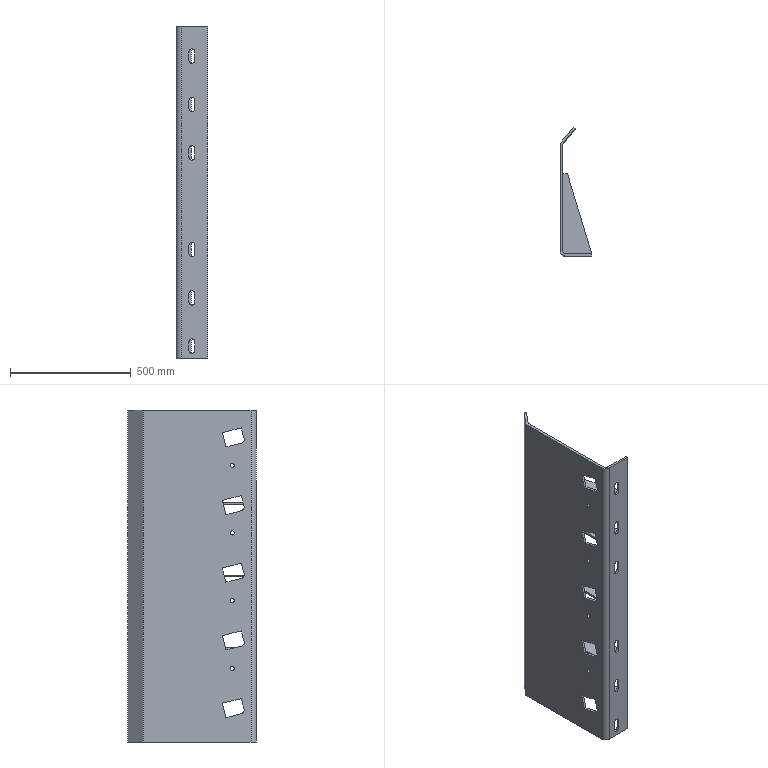Part | STEP file | Edge plate 6_Default<As machined> | 6 solids | 104 faces | box 130 x 532.359 x 1374 mm | volume 9676363 mm3 | plane 72 | cylinder 32 | commonest cylinder face diameters 24 x18 17 x8 30 x5 44 x1